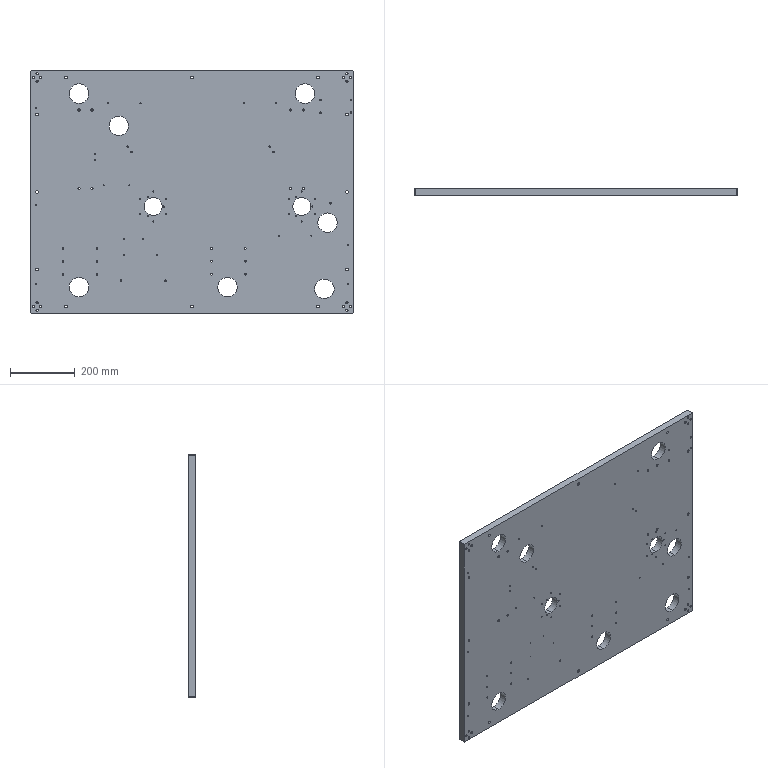Part | STEP file | 1 solid | 256 faces | box 1000 x 22 x 750 mm | volume 15887768 mm3 | cylinder 238 | plane 18 | commonest cylinder face diameters 3.3 x74 6.8 x48 5 x38 8.5 x24 15 x24 60.5 x14